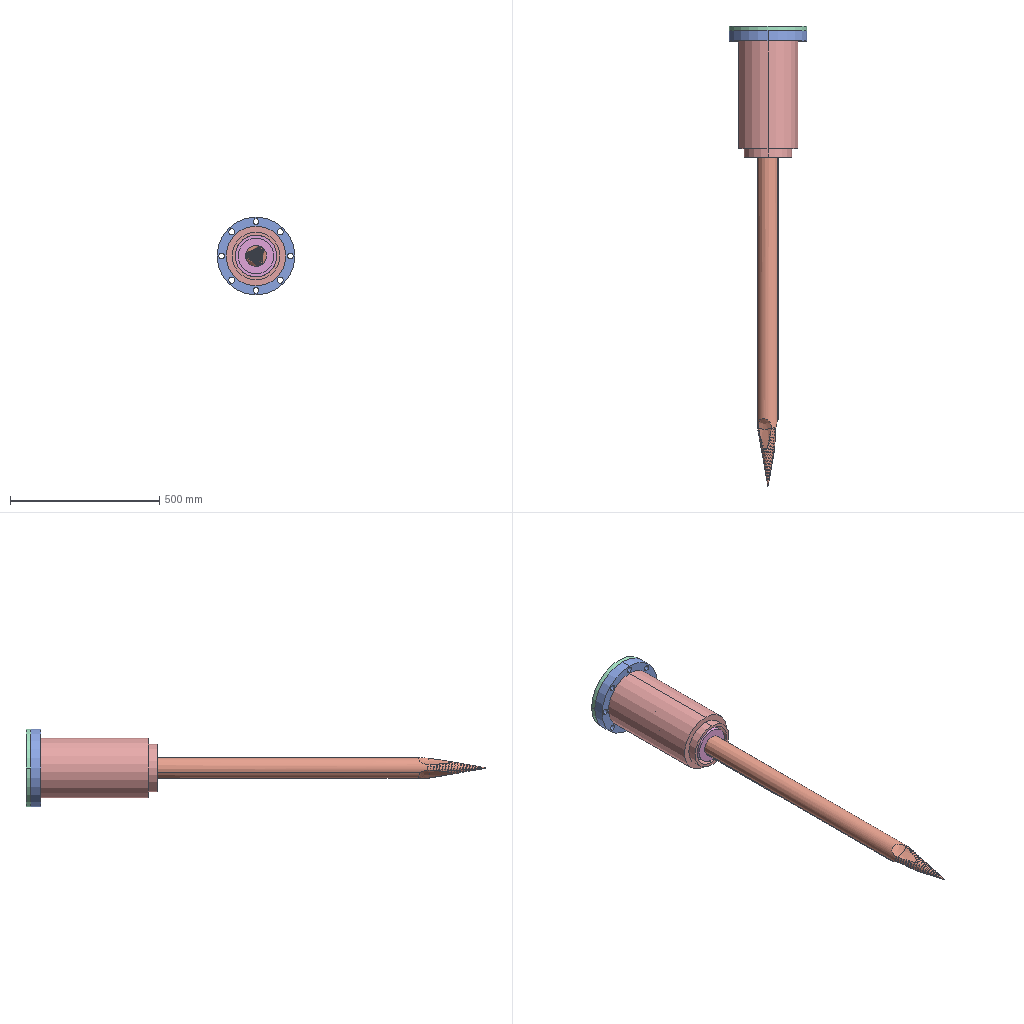Assembly | SolidWorks | 13 different items | 38 placed | box 260 x 1540 x 260 mm
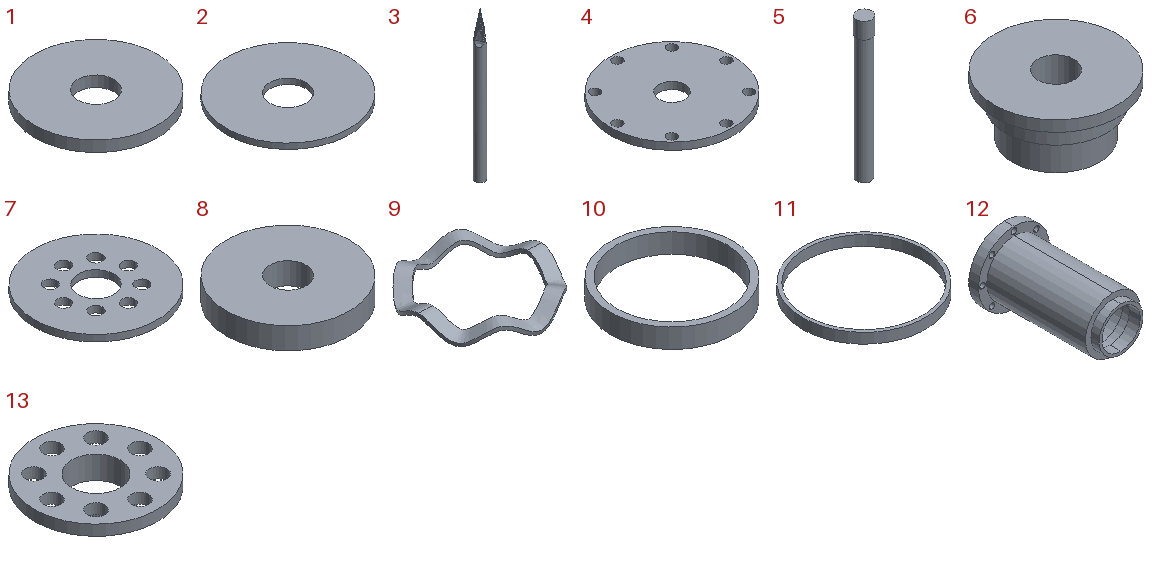Parts list (item | quantity | size | volume | features):
1 | x7 | 170 x 170 x 15 mm | 311018 mm3 | features Extrusion 1
2 | x2 | 170 x 170 x 7.5 mm | 155509 mm3 | features Cut 1, Extrusion 1
3 | x1 | 70 x 70 x 1100 mm | 2879786 mm3 | features Chamfer 2, Fillet 2, Cut 1, Extrusion 1, Helix 1, ICE 1, SweepCut 1
4 | x1 | 260 x 260 x 15 mm | 723057 mm3 | features CirPattern 1, Cut 1, Extrusion 1
5 | x1 | 55 x 55 x 509 mm | 1029553 mm3 | features Extrusion 1, ICE 1
6 | x1 | 170 x 170 x 81 mm | 1034055 mm3 | features ICE 2, Cut 1, Extrusion 1
7 | x1 | 190 x 190 x 10 mm | 234638 mm3 | features CirPattern 1, Cut 1, Extrusion 1
8 | x6 | 170 x 170 x 30 mm | 622035 mm3 | features Extrusion 1
9 | x2 | 180 x 180.809 x 25.967 mm | 56026 mm3 | features 3DProfileFeature 2, 3DSplineCurve 1, Extrusion 1, Sweep 1
10 | x7 | 190 x 190 x 30 mm | 169646 mm3 | features Extrusion 1
11 | x7 | 180 x 180 x 15 mm | 41233 mm3 | features Extrusion 1
12 | x1 | 260 x 425 x 260 mm | 2163536 mm3 | features Cut 3, ICE 2, CirPattern 1, Extrusion 1, Shell 1
13 | x1 | 140 x 140 x 26 mm | 142154 mm3 | features CirPattern 1, Cut 1, Extrusion 1, ICE 1
Mates (type | each side: item.copy, entity, surface, feature):
Concentric | 12.1 face cylinder Shell1 | 9.1 select_type:24
Coincident | 12.1 face plane Shell1 | 9.1 select_type:24
Coincident | 9.1 plane | 6.1 face plane Boss-Extrude2
Concentric | 12.1 face cylinder Boss-Extrude1 | 6.1 face cylinder Boss-Extrude2
Concentric | 6.1 face cylinder Boss-Extrude2 | 2.1 face cylinder Boss-Extrude1
Coincident | 6.1 face plane Boss-Extrude2 | 2.1 face plane Boss-Extrude1
Coincident | 2.1 face plane Boss-Extrude1 | 1.1 face plane Boss-Extrude1
Concentric | 12.1 face cylinder Boss-Extrude1 | 1.1 face cylinder Boss-Extrude1
Coincident | 1.1 face plane Boss-Extrude1 | 8.1 face plane Boss-Extrude1
Concentric | 12.1 face cylinder Boss-Extrude1 | 8.1 face cylinder Boss-Extrude1
Coincident | 1.2 face plane Boss-Extrude1 | 8.2 face plane Boss-Extrude1
Coincident | 8.1 face plane Boss-Extrude1 | 1.2 face plane Boss-Extrude1
Concentric | 12.1 face cylinder Boss-Extrude1 | 1.2 face cylinder Boss-Extrude1
Concentric | 12.1 face cylinder Boss-Extrude1 | 8.2 face cylinder Boss-Extrude1
Coincident | 8.3 face plane Boss-Extrude1 | 1.3 face plane Boss-Extrude1
Coincident | 8.2 face plane Boss-Extrude1 | 1.3 face plane Boss-Extrude1
Concentric | 12.1 face cylinder Boss-Extrude1 | 1.3 face cylinder Boss-Extrude1
Concentric | 12.1 face cylinder Boss-Extrude1 | 8.3 face cylinder Boss-Extrude1
Coincident | 8.4 face plane Boss-Extrude1 | 1.4 face plane Boss-Extrude1
Coincident | 8.3 face plane Boss-Extrude1 | 1.4 face plane Boss-Extrude1
Concentric | 12.1 face cylinder Boss-Extrude1 | 1.4 face cylinder Boss-Extrude1
Concentric | 12.1 face cylinder Boss-Extrude1 | 8.4 face cylinder Boss-Extrude1
Coincident | 8.5 face plane Boss-Extrude1 | 1.5 face plane Boss-Extrude1
Coincident | 8.4 face plane Boss-Extrude1 | 1.5 face plane Boss-Extrude1
Concentric | 12.1 face cylinder Boss-Extrude1 | 1.5 face cylinder Boss-Extrude1
Concentric | 12.1 face cylinder Boss-Extrude1 | 8.5 face cylinder Boss-Extrude1
Coincident | 8.6 face plane Boss-Extrude1 | 1.6 face plane Boss-Extrude1
Coincident | 8.5 face plane Boss-Extrude1 | 1.6 face plane Boss-Extrude1
Concentric | 12.1 face cylinder Boss-Extrude1 | 1.6 face cylinder Boss-Extrude1
Concentric | 12.1 face cylinder Boss-Extrude1 | 8.6 face cylinder Boss-Extrude1
Coincident | 8.6 face plane Boss-Extrude1 | 1.7 face plane Boss-Extrude1
Concentric | 12.1 face cylinder Boss-Extrude1 | 1.7 face cylinder Boss-Extrude1
Concentric | 12.1 face cylinder Boss-Extrude1 | 2.2 face cylinder Boss-Extrude1
Coincident | 1.7 face plane Boss-Extrude1 | 2.2 face plane Boss-Extrude1
Width | 10.1 face plane Boss-Extrude1 | 10.1 face plane Boss-Extrude1 | 1.1 face plane Boss-Extrude1 | 1.1 face plane Boss-Extrude1
Concentric | 1.1 face cylinder Boss-Extrude1 | 10.1 face cylinder Boss-Extrude1
Concentric | 12.1 face cylinder Boss-Extrude1 | 11.1 face cylinder Boss-Extrude1
Coincident | 10.1 face plane Boss-Extrude1 | 11.1 face plane Boss-Extrude1
Concentric | 12.1 face cylinder Boss-Extrude1 | 11.2 face cylinder Boss-Extrude1
Coincident | 10.1 face plane Boss-Extrude1 | 11.2 face plane Boss-Extrude1
Concentric | 12.1 face cylinder Boss-Extrude1 | 10.2 face cylinder Boss-Extrude1
Coincident | 11.2 face plane Boss-Extrude1 | 10.2 edge
Coincident | 11.3 face plane Boss-Extrude1 | 10.3 edge
Concentric | 12.1 face cylinder Boss-Extrude1 | 11.3 face cylinder Boss-Extrude1
Coincident | 10.2 face plane Boss-Extrude1 | 11.3 face plane Boss-Extrude1
Concentric | 12.1 face cylinder Boss-Extrude1 | 10.3 face cylinder Boss-Extrude1
Coincident | 11.4 face plane Boss-Extrude1 | 10.4 edge
Concentric | 1.4 face cylinder Boss-Extrude1 | 11.4 face cylinder Boss-Extrude1
Coincident | 10.3 face plane Boss-Extrude1 | 11.4 face plane Boss-Extrude1
Concentric | 12.1 face cylinder Boss-Extrude1 | 10.4 face cylinder Boss-Extrude1
Coincident | 11.5 face plane Boss-Extrude1 | 10.5 edge
Concentric | 12.1 face cylinder Boss-Extrude1 | 11.5 face cylinder Boss-Extrude1
Coincident | 10.4 face plane Boss-Extrude1 | 11.5 face plane Boss-Extrude1
Concentric | 12.1 face cylinder Boss-Extrude1 | 10.5 face cylinder Boss-Extrude1
Coincident | 11.6 face plane Boss-Extrude1 | 10.6 edge
Concentric | 12.1 face cylinder Boss-Extrude1 | 11.6 face cylinder Boss-Extrude1
Coincident | 10.5 face plane Boss-Extrude1 | 11.6 face plane Boss-Extrude1
Concentric | 12.1 face cylinder Boss-Extrude1 | 10.6 face cylinder Boss-Extrude1
Coincident | 10.6 face plane Boss-Extrude1 | 11.7 face plane Boss-Extrude1
Concentric | 12.1 face cylinder Boss-Extrude1 | 11.7 face cylinder Boss-Extrude1
Coincident | 11.7 face plane Boss-Extrude1 | 10.7 edge
Concentric | 12.1 face cylinder Boss-Extrude3 | 10.7 face cylinder Boss-Extrude1
Coincident | 2.2 face plane Boss-Extrude1 | 7.1 face plane Boss-Extrude1
Concentric | 2.2 edge | 7.1 edge
Coincident | 7.1 face plane Boss-Extrude1 | 13.1 face plane Boss-Extrude1
Concentric | 7.1 face cylinder Cut-Extrude1 | 13.1 face cylinder CirPattern1
Coincident | 7.1 face plane Boss-Extrude1 | 9.2 plane
Concentric | 13.1 edge | 9.2 select_type:24
InPlace | 2.2 face plane Boss-Extrude1 | 5.1 plane
InPlace | 12.1 face plane Boss-Extrude3 | 4.1 plane
InPlace | 6.1 face plane Boss-Extrude3 | 3.1 plane